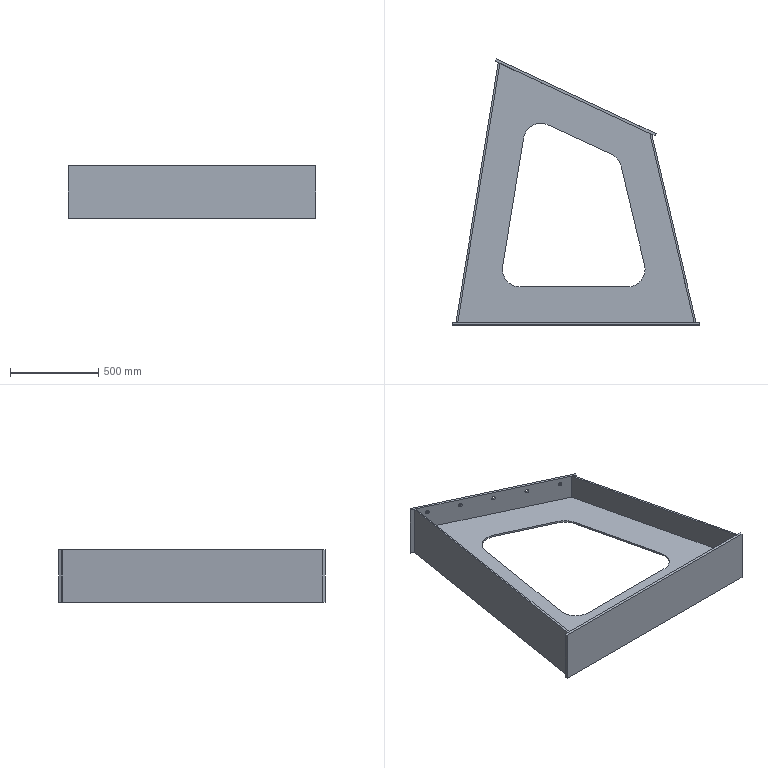Part | STEP file | Leg_Default<As machined> | 5 solids | 59 faces | box 1400 x 1507 x 300 mm | volume 26750230 mm3 | plane 34 | cylinder 25 | commonest cylinder face diameters 22 x20 200.073 x2 199.95 x1 200 x1 200.102 x1